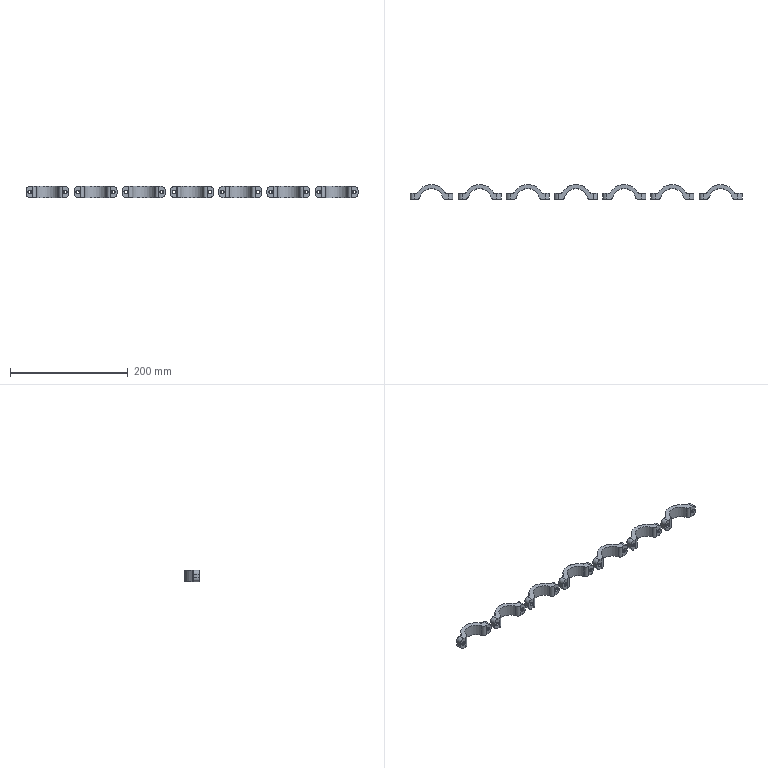CAM job | Mastercam | 3-axis milling, 5-axis milling, drilling | stock box 575 x 30 x 25 mm
Tools:
tool_number,name,type,diameter_mm,corner_radius_mm,flutes,flute_length_mm,overall_length_mm,shoulder_length_mm,holder_diameter_mm,length_offset,diameter_offset,default_rpm,default_feed_mm_min,default_plunge_mm_min,coolant
1,16 Corn cutter,end mill,16,0,4,25,50,25,50,1,1,5500,2000,2000,COOL_OFF
2,8 Finish cutter,end mill,8,0,4,25,30,25,50,2,2,5500,800,2000,COOL_OFF
3,6R0.5 Mill,bull end mill,6,0.5,4,20,20,20,50,3,3,2000,240,600,COOL_OFF
4,6 Chamfer Mill,chamfer mill,6,0,4,25,25,25,50,4,4,4167,500.04,600,COOL_OFF
5,8 Flat End Mill Rough,end mill,8,0,4,25,25,25,50,5,5,1250,150,600,COOL_OFF
6,5 Drill,drill,5,0,2,25,50,40,50,6,6,1200,144,600,COOL_OFF
7,M6 x 1 RH Tap,drill,6,0,2,24,62,24,50,7,7,1000,1000,600,COOL_OFF
8,6.8 Drill,drill,6.8,0,2,25,50,40,50,8,8,882,105.84,600,COOL_OFF
9,4 Ball Mill,ball end mill,4,2,4,20,20,20,50,9,9,3000,360,600,COOL_OFF
10,8 Drill,drill,8,0,2,25,50,40,50,10,10,750,90,600,COOL_OFF
11,6 Flat End Mill,end mill,6,0,4,20,20,20,50,11,11,1667,200.04,600,COOL_OFF
Operations:
seq,operation,operation_type,tool_number,tool_name,tool_diameter_mm,spindle_rpm,feed_mm_min,plunge_mm_min,retract_mm_min,cycle_time_s,wcs,posted,nc_file
1,Contour (2D) - [WCS: Top] - [Tplane: Top],Contour,1,16 Corn cutter,16,5000,800,2000,5000,10.269,Top,yes,.nc
2,2D High Speed (2D Dynamic Mill) - [WCS: Top] - [Tplane: Top],HighSpeed2D,1,16 Corn cutter,16,6000,4000,2000,1200,61.896,Top,yes,.nc
3,Contour (2D) - [WCS: Top] - [Tplane: Top],Contour,1,16 Corn cutter,16,3000,1000,2000,5000,5.699,Top,yes,.nc
4,Contour (Remachining) - [WCS: Top] - [Tplane: Top],Contour,2,8 Finish cutter,8,3500,800,2000,5000,123.23,Top,yes,.nc
5,Contour (2D) - [WCS: Top] - [Tplane: Top],Contour,2,8 Finish cutter,8,3500,800,2000,5000,13.213,Top,yes,.nc
6,Surface Finish Flowline - [WCS: Top] - [Tplane: Top],MultiSurfaceFinishFlowline,3,6R0.5 Mill,6,6500,4000,600,1200,26.261,Top,yes,.nc
7,Contour (2D chamfer) - [WCS: Top] - [Tplane: Top],Contour,4,6 Chamfer Mill,6,5000,1000,2000,1200,12.117,Top,yes,.nc
8,2D High Speed (2D Dynamic Mill) - [WCS: Top] - [Tplane: Plane-2],HighSpeed2D,1,16 Corn cutter,16,6000,4000,2000,1200,37.949,Top,no,
9,Contour (2D) - [WCS: Top] - [Tplane: Plane-2],Contour,1,16 Corn cutter,16,5500,800,2000,5000,8.384,Top,no,
10,Surface Finish Flowline - [WCS: Top] - [Tplane: Plane-2],MultiSurfaceFinishFlowline,3,6R0.5 Mill,6,6500,4000,600,1200,25.685,Top,no,
11,Deburr 5-axis - [WCS: Top] - [Tplane: Plane-2],459,9,4 Ball Mill,4,6000,1000,2000,1200,12.84,Top,no,
12,Transform/Translate Rectangular/Coordinate/NCI,XForm,,,,0,0,0,0,169.717,Top,yes,.nc
13,Drill/Counterbore - [WCS: Top] - [Tplane: Plane-1],Drill,4,6 Chamfer Mill,6,3000,300,600,1200,2.17,Top,no,
14,Drill/Counterbore - [WCS: Top] - [Tplane: Plane-1],Drill,6,5 Drill,5,3000,300,600,1200,7.085,Top,no,
15,Drill/Counterbore - [WCS: Top] - [Tplane: Plane-1],Drill,8,6.8 Drill,6.8,1500,150,600,1200,5.636,Top,no,
16,Tap - [WCS: Top] - [Tplane: Plane-1],Drill,7,M6 x 1 RH Tap,6,200,200,600,1200,46.67,Top,no,
17,Transform/Translate Rectangular/Coordinate/NCI,XForm,,,,0,0,0,0,123.123,Top,yes,.nc
18,Contour (2D) - [WCS: Top] - [Tplane: Top],Contour,1,16 Corn cutter,16,5000,800,2000,5000,51.047,Top,yes,.nc
19,2D High Speed (2D Dynamic Mill) - [WCS: Top] - [Tplane: Top],HighSpeed2D,1,16 Corn cutter,16,6500,4000,2000,1200,324.67,Top,yes,.nc
20,Contour (2D) - [WCS: Top] - [Tplane: Top],Contour,1,16 Corn cutter,16,3000,1000,2000,5000,5.699,Top,yes,.nc
21,Transform/Translate Rectangular/Coordinate/NCI,XForm,,,,0,0,0,0,34.197,Top,yes,.nc
22,Surface Finish Flowline - [WCS: Top] - [Tplane: Top],MultiSurfaceFinishFlowline,3,6R0.5 Mill,6,6500,4000,600,1200,12.701,Top,yes,.nc
23,Surface Finish Flowline - [WCS: Top] - [Tplane: Top],MultiSurfaceFinishFlowline,3,6R0.5 Mill,6,6500,4000,600,1200,12.701,Top,yes,.nc
24,Transform/Translate Rectangular/Coordinate/NCI,XForm,,,,0,0,0,0,152.412,Top,yes,.nc
25,Contour (Ramp) - [WCS: Top] - [Tplane: Top],Contour,5,8 Flat End Mill Rough,8,5500,2000,2000,1200,56.758,Top,yes,.nc
26,Contour (Remachining) - [WCS: Top] - [Tplane: Top],Contour,2,8 Finish cutter,8,3500,800,2000,5000,60.619,Top,yes,.nc
27,Contour (2D) - [WCS: Top] - [Tplane: Top],Contour,2,8 Finish cutter,8,3500,800,2000,5000,13.275,Top,yes,.nc
28,Transform/Translate Rectangular/Coordinate/NCI,XForm,,,,0,0,0,0,79.649,Top,yes,.nc
29,Deburr 5-axis - [WCS: Top] - [Tplane: Top],459,9,4 Ball Mill,4,6000,1000,2000,1200,13.795,Top,yes,.nc
30,Transform/Translate Rectangular/Coordinate/NCI,XForm,,,,0,0,0,0,82.773,Top,yes,.nc
31,Contour (Ramp) - [WCS: Top] - [Tplane: Top],Contour,5,8 Flat End Mill Rough,8,5500,2000,2000,1200,40.362,Top,yes,.nc
32,Drill/Counterbore - [WCS: Top] - [Tplane: Vise jaw],Drill,4,6 Chamfer Mill,6,3000,300,600,1200,2.17,Top,yes,.nc
33,Drill/Counterbore - [WCS: Top] - [Tplane: Vise jaw],Drill,10,8 Drill,8,3000,300,600,1200,6.675,Top,yes,.nc
34,Pocket (Standard) - [WCS: Top] - [Tplane: Vise jaw],Pocket,11,6 Flat End Mill,6,5000,1000,2000,1200,312.63,Top,yes,.nc
35,Pocket (Standard) - [WCS: Top] - [Tplane: Vise jaw],Pocket,11,6 Flat End Mill,6,5000,600,2000,1200,47.074,Top,yes,.nc
36,Contour (2D) - [WCS: Top] - [Tplane: Vise jaw],Contour,11,6 Flat End Mill,6,5000,600,2000,1200,18.925,Top,yes,.nc
37,Contour (2D) - [WCS: Top] - [Tplane: Top-1],Contour,1,16 Corn cutter,16,3000,1000,2000,5000,5.758,Top,yes,.nc